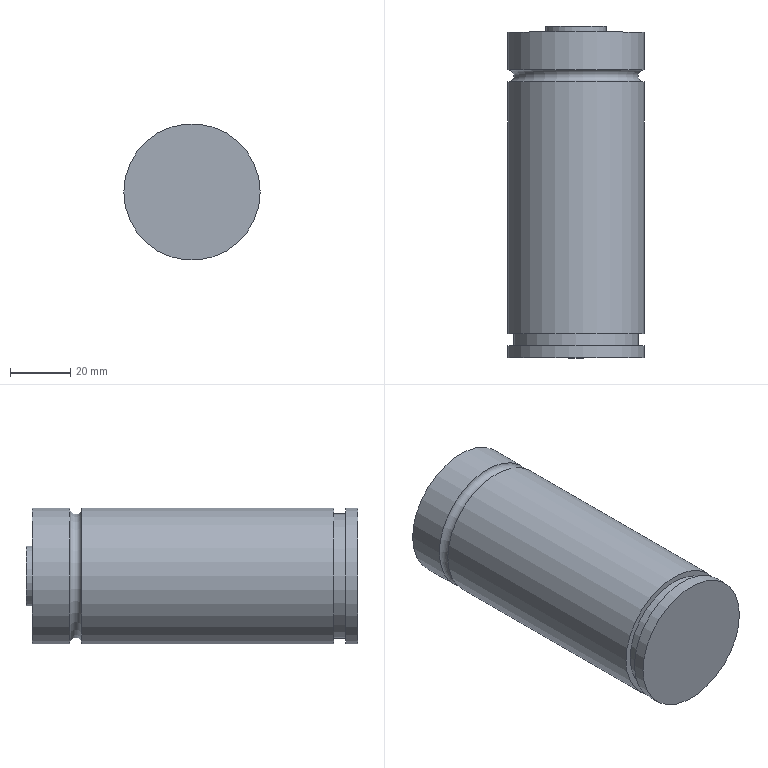Part | NX | features MAIN_BODY 2 | 1 solid | 11 faces | box 45.2 x 110 x 45.2 mm | volume 171981 mm3 | cylinder 5 | plane 5 | torus 1 | commonest cylinder face diameters 45.2 x3 20 x1 41.2 x1
STEP:
#1=CARTESIAN_POINT('',(-551.6,-677.,-215.));
#2=VERTEX_POINT('',#1);
#3=CARTESIAN_POINT('',(-529.,-677.,-215.));
#4=DIRECTION('',(0.,1.,0.));
#5=DIRECTION('',(-1.,0.,0.));
#6=AXIS2_PLACEMENT_3D('',#3,#4,#5);
#7=CIRCLE('',#6,22.6);
#8=EDGE_CURVE('',#2,#2,#7,.F.);
#9=ORIENTED_EDGE('',*,*,#8,.F.);
#10=EDGE_LOOP('',(#9));
#11=FACE_BOUND('',#10,.T.);
#12=CARTESIAN_POINT('',(-551.6,-593.5,-215.));
#13=VERTEX_POINT('',#12);
#14=CARTESIAN_POINT('',(-529.,-593.5,-215.));
#15=DIRECTION('',(0.,1.,0.));
#16=DIRECTION('',(-1.,0.,0.));
#17=AXIS2_PLACEMENT_3D('',#14,#15,#16);
#18=CIRCLE('',#17,22.6);
#19=EDGE_CURVE('',#13,#13,#18,.T.);
#20=ORIENTED_EDGE('',*,*,#19,.F.);
#21=EDGE_LOOP('',(#20));
#22=FACE_BOUND('',#21,.T.);
#23=CARTESIAN_POINT('',(-529.,-577.,-215.));
#24=DIRECTION('',(0.,-1.,0.));
#25=DIRECTION('',(-1.,0.,0.));
#26=AXIS2_PLACEMENT_3D('',#23,#24,#25);
#27=CYLINDRICAL_SURFACE('',#26,22.6);
#28=ADVANCED_FACE('',(#11,#22),#27,.T.);
#29=CARTESIAN_POINT('',(-506.4,-577.,-215.));
#30=VERTEX_POINT('',#29);
#31=CARTESIAN_POINT('',(-529.,-577.,-215.));
#32=DIRECTION('',(0.,-1.,0.));
#33=DIRECTION('',(1.,0.,0.));
#34=AXIS2_PLACEMENT_3D('',#31,#32,#33);
#35=CIRCLE('',#34,22.6);
#36=EDGE_CURVE('',#30,#30,#35,.T.);
#37=ORIENTED_EDGE('',*,*,#36,.F.);
#38=EDGE_LOOP('',(#37));
#39=FACE_BOUND('',#38,.T.);
#40=CARTESIAN_POINT('',(-519.,-577.,-215.));
#41=VERTEX_POINT('',#40);
#42=CARTESIAN_POINT('',(-529.,-577.,-215.));
#43=DIRECTION('',(0.,-1.,0.));
#44=DIRECTION('',(1.,0.,0.));
#45=AXIS2_PLACEMENT_3D('',#42,#43,#44);
#46=CIRCLE('',#45,10.);
#47=EDGE_CURVE('',#41,#41,#46,.T.);
#48=ORIENTED_EDGE('',*,*,#47,.T.);
#49=EDGE_LOOP('',(#48));
#50=FACE_BOUND('',#49,.T.);
#51=CARTESIAN_POINT('',(-529.,-577.,-215.));
#52=DIRECTION('',(0.,1.,0.));
#53=DIRECTION('',(1.,0.,0.));
#54=AXIS2_PLACEMENT_3D('',#51,#52,#53);
#55=PLANE('',#54);
#56=ADVANCED_FACE('',(#39,#50),#55,.T.);
#57=CARTESIAN_POINT('',(-551.6,-589.5,-215.));
#58=VERTEX_POINT('',#57);
#59=CARTESIAN_POINT('',(-529.,-589.5,-215.));
#60=DIRECTION('',(0.,1.,0.));
#61=DIRECTION('',(-1.,0.,0.));
#62=AXIS2_PLACEMENT_3D('',#59,#60,#61);
#63=CIRCLE('',#62,22.6);
#64=EDGE_CURVE('',#58,#58,#63,.F.);
#65=ORIENTED_EDGE('',*,*,#64,.F.);
#66=EDGE_LOOP('',(#65));
#67=FACE_BOUND('',#66,.T.);
#68=ORIENTED_EDGE('',*,*,#36,.T.);
#69=EDGE_LOOP('',(#68));
#70=FACE_BOUND('',#69,.T.);
#71=CARTESIAN_POINT('',(-529.,-577.,-215.));
#72=DIRECTION('',(0.,-1.,0.));
#73=DIRECTION('',(-1.,0.,0.));
#74=AXIS2_PLACEMENT_3D('',#71,#72,#73);
#75=CYLINDRICAL_SURFACE('',#74,22.6);
#76=ADVANCED_FACE('',(#67,#70),#75,.T.);
#77=CARTESIAN_POINT('',(-519.,-575.,-215.));
#78=VERTEX_POINT('',#77);
#79=CARTESIAN_POINT('',(-529.,-575.,-215.));
#80=DIRECTION('',(0.,-1.,0.));
#81=DIRECTION('',(1.,0.,0.));
#82=AXIS2_PLACEMENT_3D('',#79,#80,#81);
#83=CIRCLE('',#82,10.);
#84=EDGE_CURVE('',#78,#78,#83,.T.);
#85=ORIENTED_EDGE('',*,*,#84,.T.);
#86=EDGE_LOOP('',(#85));
#87=FACE_BOUND('',#86,.T.);
#88=ORIENTED_EDGE('',*,*,#47,.F.);
#89=EDGE_LOOP('',(#88));
#90=FACE_BOUND('',#89,.T.);
#91=CARTESIAN_POINT('',(-529.,-575.,-215.));
#92=DIRECTION('',(0.,-1.,0.));
#93=DIRECTION('',(-1.,0.,0.));
#94=AXIS2_PLACEMENT_3D('',#91,#92,#93);
#95=CYLINDRICAL_SURFACE('',#94,10.);
#96=ADVANCED_FACE('',(#87,#90),#95,.T.);
#97=ORIENTED_EDGE('',*,*,#84,.F.);
#98=EDGE_LOOP('',(#97));
#99=FACE_BOUND('',#98,.T.);
#100=CARTESIAN_POINT('',(-529.,-575.,-215.));
#101=DIRECTION('',(0.,1.,0.));
#102=DIRECTION('',(1.,0.,0.));
#103=AXIS2_PLACEMENT_3D('',#100,#101,#102);
#104=PLANE('',#103);
#105=ADVANCED_FACE('',(#99),#104,.T.);
#106=ORIENTED_EDGE('',*,*,#64,.T.);
#107=EDGE_LOOP('',(#106));
#108=FACE_BOUND('',#107,.T.);
#109=ORIENTED_EDGE('',*,*,#19,.T.);
#110=EDGE_LOOP('',(#109));
#111=FACE_BOUND('',#110,.T.);
#112=CARTESIAN_POINT('',(-529.,-591.5,-215.));
#113=DIRECTION('',(0.,-1.,0.));
#114=DIRECTION('',(-1.,0.,0.));
#115=AXIS2_PLACEMENT_3D('',#112,#113,#114);
#116=TOROIDAL_SURFACE('',#115,22.6,2.);
#117=ADVANCED_FACE('',(#108,#111),#116,.F.);
#118=CARTESIAN_POINT('',(-508.4,-677.,-215.));
#119=VERTEX_POINT('',#118);
#120=CARTESIAN_POINT('',(-529.,-677.,-215.));
#121=DIRECTION('',(0.,-1.,0.));
#122=DIRECTION('',(1.,0.,0.));
#123=AXIS2_PLACEMENT_3D('',#120,#121,#122);
#124=CIRCLE('',#123,20.6);
#125=EDGE_CURVE('',#119,#119,#124,.T.);
#126=ORIENTED_EDGE('',*,*,#125,.F.);
#127=EDGE_LOOP('',(#126));
#128=FACE_BOUND('',#127,.T.);
#129=ORIENTED_EDGE('',*,*,#8,.T.);
#130=EDGE_LOOP('',(#129));
#131=FACE_BOUND('',#130,.T.);
#132=CARTESIAN_POINT('',(-529.,-677.,-215.));
#133=DIRECTION('',(0.,-1.,0.));
#134=DIRECTION('',(-1.,0.,0.));
#135=AXIS2_PLACEMENT_3D('',#132,#133,#134);
#136=PLANE('',#135);
#137=ADVANCED_FACE('',(#128,#131),#136,.T.);
#138=CARTESIAN_POINT('',(-508.4,-681.,-215.));
#139=VERTEX_POINT('',#138);
#140=CARTESIAN_POINT('',(-529.,-681.,-215.));
#141=DIRECTION('',(0.,-1.,0.));
#142=DIRECTION('',(1.,0.,0.));
#143=AXIS2_PLACEMENT_3D('',#140,#141,#142);
#144=CIRCLE('',#143,20.6);
#145=EDGE_CURVE('',#139,#139,#144,.T.);
#146=ORIENTED_EDGE('',*,*,#145,.T.);
#147=EDGE_LOOP('',(#146));
#148=FACE_BOUND('',#147,.T.);
#149=CARTESIAN_POINT('',(-551.6,-681.,-215.));
#150=VERTEX_POINT('',#149);
#151=CARTESIAN_POINT('',(-529.,-681.,-215.));
#152=DIRECTION('',(0.,1.,0.));
#153=DIRECTION('',(-1.,0.,0.));
#154=AXIS2_PLACEMENT_3D('',#151,#152,#153);
#155=CIRCLE('',#154,22.6);
#156=EDGE_CURVE('',#150,#150,#155,.T.);
#157=ORIENTED_EDGE('',*,*,#156,.T.);
#158=EDGE_LOOP('',(#157));
#159=FACE_BOUND('',#158,.T.);
#160=CARTESIAN_POINT('',(-529.,-681.,-215.));
#161=DIRECTION('',(0.,-1.,0.));
#162=DIRECTION('',(-1.,0.,0.));
#163=AXIS2_PLACEMENT_3D('',#160,#161,#162);
#164=PLANE('',#163);
#165=ADVANCED_FACE('',(#148,#159),#164,.F.);
#166=ORIENTED_EDGE('',*,*,#125,.T.);
#167=EDGE_LOOP('',(#166));
#168=FACE_BOUND('',#167,.T.);
#169=ORIENTED_EDGE('',*,*,#145,.F.);
#170=EDGE_LOOP('',(#169));
#171=FACE_BOUND('',#170,.T.);
#172=CARTESIAN_POINT('',(-529.,-681.,-215.));
#173=DIRECTION('',(0.,1.,0.));
#174=DIRECTION('',(1.,0.,0.));
#175=AXIS2_PLACEMENT_3D('',#172,#173,#174);
#176=CYLINDRICAL_SURFACE('',#175,20.6);
#177=ADVANCED_FACE('',(#168,#171),#176,.T.);
#178=CARTESIAN_POINT('',(-506.4,-685.,-215.));
#179=VERTEX_POINT('',#178);
#180=CARTESIAN_POINT('',(-529.,-685.,-215.));
#181=DIRECTION('',(0.,-1.,0.));
#182=DIRECTION('',(1.,0.,0.));
#183=AXIS2_PLACEMENT_3D('',#180,#181,#182);
#184=CIRCLE('',#183,22.6);
#185=EDGE_CURVE('',#179,#179,#184,.T.);
#186=ORIENTED_EDGE('',*,*,#185,.T.);
#187=EDGE_LOOP('',(#186));
#188=FACE_BOUND('',#187,.T.);
#189=CARTESIAN_POINT('',(-529.,-685.,-215.));
#190=DIRECTION('',(0.,1.,0.));
#191=DIRECTION('',(1.,0.,0.));
#192=AXIS2_PLACEMENT_3D('',#189,#190,#191);
#193=PLANE('',#192);
#194=ADVANCED_FACE('',(#188),#193,.F.);
#195=ORIENTED_EDGE('',*,*,#156,.F.);
#196=EDGE_LOOP('',(#195));
#197=FACE_BOUND('',#196,.T.);
#198=ORIENTED_EDGE('',*,*,#185,.F.);
#199=EDGE_LOOP('',(#198));
#200=FACE_BOUND('',#199,.T.);
#201=CARTESIAN_POINT('',(-529.,-577.,-215.));
#202=DIRECTION('',(0.,-1.,0.));
#203=DIRECTION('',(-1.,0.,0.));
#204=AXIS2_PLACEMENT_3D('',#201,#202,#203);
#205=CYLINDRICAL_SURFACE('',#204,22.6);
#206=ADVANCED_FACE('',(#197,#200),#205,.T.);
#207=CLOSED_SHELL('',(#28,#56,#76,#96,#105,#117,#137,#165,#177,#194,#206));
#208=MANIFOLD_SOLID_BREP('',#207);
#209=(LENGTH_UNIT()NAMED_UNIT(*)SI_UNIT(.MILLI.,.METRE.));
#210=UNCERTAINTY_MEASURE_WITH_UNIT(LENGTH_MEASURE(0.00001),#209,'','');
#211=(NAMED_UNIT(*)PLANE_ANGLE_UNIT()SI_UNIT($,.RADIAN.));
#212=(NAMED_UNIT(*)SI_UNIT($,.STERADIAN.)SOLID_ANGLE_UNIT());
#213=(GEOMETRIC_REPRESENTATION_CONTEXT(3)GLOBAL_UNCERTAINTY_ASSIGNED_CONTEXT((#210))GLOBAL_UNIT_ASSIGNED_CONTEXT((#209,#211,#212))REPRESENTATION_CONTEXT('',''));
#214=ADVANCED_BREP_SHAPE_REPRESENTATION('',(#208),#213);